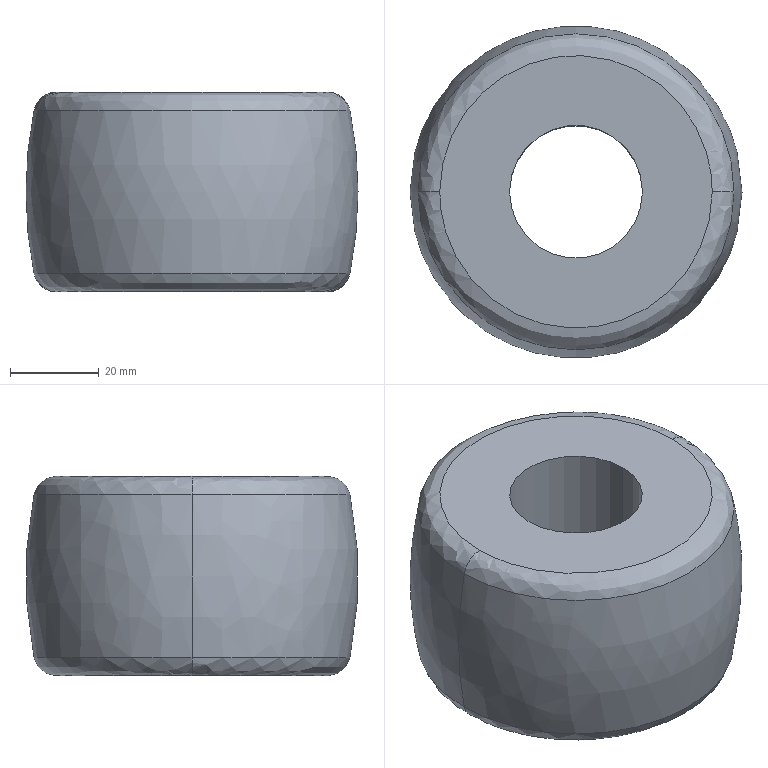Part | STEP file | CDAN75-Mw | 1 solid | 10 faces | box 75 x 74.925 x 45 mm | volume 156321 mm3 | spline 6 | cylinder 2 | plane 2 | commonest cylinder face diameters 30 x2
STEP:
#1=CARTESIAN_POINT('',(0.,0.,0.));
#2=DIRECTION('',(0.,0.,1.));
#3=DIRECTION('',(1.,0.,0.));
#4=AXIS2_PLACEMENT_3D('',#1,#2,#3);
#5=CARTESIAN_POINT('',(-20.313,-59.,18.472));
#6=VERTEX_POINT('',#5);
#7=CARTESIAN_POINT('',(-91.687,-59.,18.472));
#8=VERTEX_POINT('',#7);
#9=CARTESIAN_POINT('',(-56.,-59.,18.472));
#10=DIRECTION('',(0.,0.,-1.));
#11=DIRECTION('',(1.,0.,0.));
#12=AXIS2_PLACEMENT_3D('',#9,#10,#11);
#13=CIRCLE('',#12,35.687);
#14=CARTESIAN_POINT('',(-91.687,-59.,18.472));
#15=CARTESIAN_POINT('',(-91.687,-130.374,18.472));
#16=CARTESIAN_POINT('',(-20.313,-130.374,18.472));
#17=CARTESIAN_POINT('',(-20.313,-59.,18.472));
#18=CARTESIAN_POINT('',(-94.112,-59.,6.237));
#19=CARTESIAN_POINT('',(-94.112,-135.224,6.237));
#20=CARTESIAN_POINT('',(-17.888,-135.224,6.237));
#21=CARTESIAN_POINT('',(-17.888,-59.,6.237));
#22=CARTESIAN_POINT('',(-94.112,-59.,-6.237));
#23=CARTESIAN_POINT('',(-94.112,-135.224,-6.237));
#24=CARTESIAN_POINT('',(-17.888,-135.224,-6.237));
#25=CARTESIAN_POINT('',(-17.888,-59.,-6.237));
#26=CARTESIAN_POINT('',(-91.687,-59.,-18.472));
#27=CARTESIAN_POINT('',(-91.687,-130.374,-18.472));
#28=CARTESIAN_POINT('',(-20.313,-130.374,-18.472));
#29=CARTESIAN_POINT('',(-20.313,-59.,-18.472));
#30=(BOUNDED_SURFACE()B_SPLINE_SURFACE(3,3,((#14,#15,#16,#17),(#18,#19,#20,#21),(#22,#23,#24,#25),(#26,#27,#28,#29)),.UNSPECIFIED.,.F.,.F.,.F.)B_SPLINE_SURFACE_WITH_KNOTS((4,4),(4,4),(0.,1.),(0.,1.),.PIECEWISE_BEZIER_KNOTS.)GEOMETRIC_REPRESENTATION_ITEM()RATIONAL_B_SPLINE_SURFACE(((1.,0.3333,0.3333,1.),(0.9873,0.3291,0.3291,0.9873),(0.9873,0.3291,0.3291,0.9873),(1.,0.3333,0.3333,1.)))REPRESENTATION_ITEM('')SURFACE());
#31=CARTESIAN_POINT('',(0.,1.));
#32=CARTESIAN_POINT('',(0.,0.9763));
#33=CARTESIAN_POINT('',(0.,0.9319));
#34=CARTESIAN_POINT('',(0.,0.8733));
#35=CARTESIAN_POINT('',(0.,0.8206));
#36=CARTESIAN_POINT('',(0.,0.7724));
#37=CARTESIAN_POINT('',(0.,0.7279));
#38=CARTESIAN_POINT('',(0.,0.6861));
#39=CARTESIAN_POINT('',(0.,0.6465));
#40=CARTESIAN_POINT('',(0.,0.6086));
#41=CARTESIAN_POINT('',(0.,0.5718));
#42=CARTESIAN_POINT('',(0.,0.5357));
#43=CARTESIAN_POINT('',(0.,0.5));
#44=CARTESIAN_POINT('',(0.,0.4643));
#45=CARTESIAN_POINT('',(0.,0.4282));
#46=CARTESIAN_POINT('',(0.,0.3914));
#47=CARTESIAN_POINT('',(0.,0.3535));
#48=CARTESIAN_POINT('',(0.,0.3139));
#49=CARTESIAN_POINT('',(0.,0.2721));
#50=CARTESIAN_POINT('',(0.,0.2276));
#51=CARTESIAN_POINT('',(0.,0.1794));
#52=CARTESIAN_POINT('',(0.,0.1267));
#53=CARTESIAN_POINT('',(0.,0.06805));
#54=CARTESIAN_POINT('',(0.,0.02375));
#55=CARTESIAN_POINT('',(0.,0.));
#56=B_SPLINE_CURVE_WITH_KNOTS('',3,(#31,#32,#33,#34,#35,#36,#37,#38,#39,#40,#41,#42,#43,#44,#45,#46,#47,#48,#49,#50,#51,#52,#53,#54,#55),.UNSPECIFIED.,.F.,.F.,(4,1,1,1,1,1,1,1,1,1,1,1,1,1,1,1,1,1,1,1,1,1,4),(0.,0.1428,0.2856,0.4284,0.5712,0.714,0.8568,0.9996,1.142,1.285,1.428,1.571,1.714,1.856,1.999,2.142,2.285,2.428,2.57,2.713,2.856,2.999,3.142),.QUASI_UNIFORM_KNOTS.);
#57=(GEOMETRIC_REPRESENTATION_CONTEXT(2)PARAMETRIC_REPRESENTATION_CONTEXT()REPRESENTATION_CONTEXT('',''));
#58=DEFINITIONAL_REPRESENTATION('',(#56),#57);
#59=PCURVE('',#30,#58);
#60=CARTESIAN_POINT('',(-86.782,-59.,22.5));
#61=CARTESIAN_POINT('',(-86.782,-120.564,22.5));
#62=CARTESIAN_POINT('',(-25.218,-120.564,22.5));
#63=CARTESIAN_POINT('',(-25.218,-59.,22.5));
#64=CARTESIAN_POINT('',(-89.275,-59.,22.5));
#65=CARTESIAN_POINT('',(-89.275,-125.551,22.5));
#66=CARTESIAN_POINT('',(-22.725,-125.551,22.5));
#67=CARTESIAN_POINT('',(-22.725,-59.,22.5));
#68=CARTESIAN_POINT('',(-91.202,-59.,20.918));
#69=CARTESIAN_POINT('',(-91.202,-129.404,20.918));
#70=CARTESIAN_POINT('',(-20.798,-129.404,20.918));
#71=CARTESIAN_POINT('',(-20.798,-59.,20.918));
#72=CARTESIAN_POINT('',(-91.687,-59.,18.472));
#73=CARTESIAN_POINT('',(-91.687,-130.374,18.472));
#74=CARTESIAN_POINT('',(-20.313,-130.374,18.472));
#75=CARTESIAN_POINT('',(-20.313,-59.,18.472));
#76=(BOUNDED_SURFACE()B_SPLINE_SURFACE(3,3,((#60,#61,#62,#63),(#64,#65,#66,#67),(#68,#69,#70,#71),(#72,#73,#74,#75)),.UNSPECIFIED.,.F.,.F.,.F.)B_SPLINE_SURFACE_WITH_KNOTS((4,4),(4,4),(0.,1.),(0.,1.),.PIECEWISE_BEZIER_KNOTS.)GEOMETRIC_REPRESENTATION_ITEM()RATIONAL_B_SPLINE_SURFACE(((1.,0.3333,0.3333,1.),(0.8485,0.2828,0.2828,0.8485),(0.8485,0.2828,0.2828,0.8485),(1.,0.3333,0.3333,1.)))REPRESENTATION_ITEM('')SURFACE());
#77=CARTESIAN_POINT('',(1.,1.));
#78=CARTESIAN_POINT('',(1.,0.9763));
#79=CARTESIAN_POINT('',(1.,0.9319));
#80=CARTESIAN_POINT('',(1.,0.8733));
#81=CARTESIAN_POINT('',(1.,0.8206));
#82=CARTESIAN_POINT('',(1.,0.7724));
#83=CARTESIAN_POINT('',(1.,0.7279));
#84=CARTESIAN_POINT('',(1.,0.6861));
#85=CARTESIAN_POINT('',(1.,0.6465));
#86=CARTESIAN_POINT('',(1.,0.6086));
#87=CARTESIAN_POINT('',(1.,0.5718));
#88=CARTESIAN_POINT('',(1.,0.5357));
#89=CARTESIAN_POINT('',(1.,0.5));
#90=CARTESIAN_POINT('',(1.,0.4643));
#91=CARTESIAN_POINT('',(1.,0.4282));
#92=CARTESIAN_POINT('',(1.,0.3914));
#93=CARTESIAN_POINT('',(1.,0.3535));
#94=CARTESIAN_POINT('',(1.,0.3139));
#95=CARTESIAN_POINT('',(1.,0.2721));
#96=CARTESIAN_POINT('',(1.,0.2276));
#97=CARTESIAN_POINT('',(1.,0.1794));
#98=CARTESIAN_POINT('',(1.,0.1267));
#99=CARTESIAN_POINT('',(1.,0.06805));
#100=CARTESIAN_POINT('',(1.,0.02375));
#101=CARTESIAN_POINT('',(1.,0.));
#102=B_SPLINE_CURVE_WITH_KNOTS('',3,(#77,#78,#79,#80,#81,#82,#83,#84,#85,#86,#87,#88,#89,#90,#91,#92,#93,#94,#95,#96,#97,#98,#99,#100,#101),.UNSPECIFIED.,.F.,.F.,(4,1,1,1,1,1,1,1,1,1,1,1,1,1,1,1,1,1,1,1,1,1,4),(0.,0.1428,0.2856,0.4284,0.5712,0.714,0.8568,0.9996,1.142,1.285,1.428,1.571,1.714,1.856,1.999,2.142,2.285,2.428,2.57,2.713,2.856,2.999,3.142),.QUASI_UNIFORM_KNOTS.);
#103=(GEOMETRIC_REPRESENTATION_CONTEXT(2)PARAMETRIC_REPRESENTATION_CONTEXT()REPRESENTATION_CONTEXT('',''));
#104=DEFINITIONAL_REPRESENTATION('',(#102),#103);
#105=PCURVE('',#76,#104);
#106=SURFACE_CURVE('',#13,(#59,#105),.PCURVE_S1.);
#107=EDGE_CURVE('',#6,#8,#106,.T.);
#108=ORIENTED_EDGE('',*,*,#107,.T.);
#109=CARTESIAN_POINT('',(-91.687,-59.,-18.472));
#110=VERTEX_POINT('',#109);
#111=CARTESIAN_POINT('',(1.5,-59.,0.));
#112=DIRECTION('',(0.,-1.,0.));
#113=DIRECTION('',(-1.,0.,0.));
#114=AXIS2_PLACEMENT_3D('',#111,#112,#113);
#115=CIRCLE('',#114,95.);
#116=CARTESIAN_POINT('',(0.,0.));
#117=CARTESIAN_POINT('',(0.01525,0.));
#118=CARTESIAN_POINT('',(0.04572,0.));
#119=CARTESIAN_POINT('',(0.09135,0.));
#120=CARTESIAN_POINT('',(0.1369,0.));
#121=CARTESIAN_POINT('',(0.1824,0.));
#122=CARTESIAN_POINT('',(0.2279,0.));
#123=CARTESIAN_POINT('',(0.2733,0.));
#124=CARTESIAN_POINT('',(0.3187,0.));
#125=CARTESIAN_POINT('',(0.364,0.));
#126=CARTESIAN_POINT('',(0.4094,0.));
#127=CARTESIAN_POINT('',(0.4547,0.));
#128=CARTESIAN_POINT('',(0.5,0.));
#129=CARTESIAN_POINT('',(0.5453,0.));
#130=CARTESIAN_POINT('',(0.5906,0.));
#131=CARTESIAN_POINT('',(0.636,0.));
#132=CARTESIAN_POINT('',(0.6813,0.));
#133=CARTESIAN_POINT('',(0.7267,0.));
#134=CARTESIAN_POINT('',(0.7721,0.));
#135=CARTESIAN_POINT('',(0.8176,0.));
#136=CARTESIAN_POINT('',(0.8631,0.));
#137=CARTESIAN_POINT('',(0.9086,0.));
#138=CARTESIAN_POINT('',(0.9543,0.));
#139=CARTESIAN_POINT('',(0.9848,0.));
#140=CARTESIAN_POINT('',(1.,0.));
#141=B_SPLINE_CURVE_WITH_KNOTS('',3,(#116,#117,#118,#119,#120,#121,#122,#123,#124,#125,#126,#127,#128,#129,#130,#131,#132,#133,#134,#135,#136,#137,#138,#139,#140),.UNSPECIFIED.,.F.,.F.,(4,1,1,1,1,1,1,1,1,1,1,1,1,1,1,1,1,1,1,1,1,1,4),(6.087,6.105,6.123,6.141,6.159,6.176,6.194,6.212,6.23,6.248,6.265,6.283,6.301,6.319,6.337,6.354,6.372,6.39,6.408,6.426,6.443,6.461,6.479),.QUASI_UNIFORM_KNOTS.);
#142=(GEOMETRIC_REPRESENTATION_CONTEXT(2)PARAMETRIC_REPRESENTATION_CONTEXT()REPRESENTATION_CONTEXT('',''));
#143=DEFINITIONAL_REPRESENTATION('',(#141),#142);
#144=PCURVE('',#30,#143);
#145=CARTESIAN_POINT('',(-20.313,-59.,18.472));
#146=CARTESIAN_POINT('',(-20.313,12.374,18.472));
#147=CARTESIAN_POINT('',(-91.687,12.374,18.472));
#148=CARTESIAN_POINT('',(-91.687,-59.,18.472));
#149=CARTESIAN_POINT('',(-17.888,-59.,6.237));
#150=CARTESIAN_POINT('',(-17.888,17.224,6.237));
#151=CARTESIAN_POINT('',(-94.112,17.224,6.237));
#152=CARTESIAN_POINT('',(-94.112,-59.,6.237));
#153=CARTESIAN_POINT('',(-17.888,-59.,-6.237));
#154=CARTESIAN_POINT('',(-17.888,17.224,-6.237));
#155=CARTESIAN_POINT('',(-94.112,17.224,-6.237));
#156=CARTESIAN_POINT('',(-94.112,-59.,-6.237));
#157=CARTESIAN_POINT('',(-20.313,-59.,-18.472));
#158=CARTESIAN_POINT('',(-20.313,12.374,-18.472));
#159=CARTESIAN_POINT('',(-91.687,12.374,-18.472));
#160=CARTESIAN_POINT('',(-91.687,-59.,-18.472));
#161=(BOUNDED_SURFACE()B_SPLINE_SURFACE(3,3,((#145,#146,#147,#148),(#149,#150,#151,#152),(#153,#154,#155,#156),(#157,#158,#159,#160)),.UNSPECIFIED.,.F.,.F.,.F.)B_SPLINE_SURFACE_WITH_KNOTS((4,4),(4,4),(0.,1.),(0.,1.),.PIECEWISE_BEZIER_KNOTS.)GEOMETRIC_REPRESENTATION_ITEM()RATIONAL_B_SPLINE_SURFACE(((1.,0.3333,0.3333,1.),(0.9873,0.3291,0.3291,0.9873),(0.9873,0.3291,0.3291,0.9873),(1.,0.3333,0.3333,1.)))REPRESENTATION_ITEM('')SURFACE());
#162=CARTESIAN_POINT('',(0.,1.));
#163=CARTESIAN_POINT('',(0.01525,1.));
#164=CARTESIAN_POINT('',(0.04572,1.));
#165=CARTESIAN_POINT('',(0.09135,1.));
#166=CARTESIAN_POINT('',(0.1369,1.));
#167=CARTESIAN_POINT('',(0.1824,1.));
#168=CARTESIAN_POINT('',(0.2279,1.));
#169=CARTESIAN_POINT('',(0.2733,1.));
#170=CARTESIAN_POINT('',(0.3187,1.));
#171=CARTESIAN_POINT('',(0.364,1.));
#172=CARTESIAN_POINT('',(0.4094,1.));
#173=CARTESIAN_POINT('',(0.4547,1.));
#174=CARTESIAN_POINT('',(0.5,1.));
#175=CARTESIAN_POINT('',(0.5453,1.));
#176=CARTESIAN_POINT('',(0.5906,1.));
#177=CARTESIAN_POINT('',(0.636,1.));
#178=CARTESIAN_POINT('',(0.6813,1.));
#179=CARTESIAN_POINT('',(0.7267,1.));
#180=CARTESIAN_POINT('',(0.7721,1.));
#181=CARTESIAN_POINT('',(0.8176,1.));
#182=CARTESIAN_POINT('',(0.8631,1.));
#183=CARTESIAN_POINT('',(0.9086,1.));
#184=CARTESIAN_POINT('',(0.9543,1.));
#185=CARTESIAN_POINT('',(0.9848,1.));
#186=CARTESIAN_POINT('',(1.,1.));
#187=B_SPLINE_CURVE_WITH_KNOTS('',3,(#162,#163,#164,#165,#166,#167,#168,#169,#170,#171,#172,#173,#174,#175,#176,#177,#178,#179,#180,#181,#182,#183,#184,#185,#186),.UNSPECIFIED.,.F.,.F.,(4,1,1,1,1,1,1,1,1,1,1,1,1,1,1,1,1,1,1,1,1,1,4),(6.087,6.105,6.123,6.141,6.159,6.176,6.194,6.212,6.23,6.248,6.265,6.283,6.301,6.319,6.337,6.354,6.372,6.39,6.408,6.426,6.443,6.461,6.479),.QUASI_UNIFORM_KNOTS.);
#188=(GEOMETRIC_REPRESENTATION_CONTEXT(2)PARAMETRIC_REPRESENTATION_CONTEXT()REPRESENTATION_CONTEXT('',''));
#189=DEFINITIONAL_REPRESENTATION('',(#187),#188);
#190=PCURVE('',#161,#189);
#191=SURFACE_CURVE('',#115,(#144,#190),.PCURVE_S1.);
#192=EDGE_CURVE('',#8,#110,#191,.T.);
#193=ORIENTED_EDGE('',*,*,#192,.T.);
#194=CARTESIAN_POINT('',(-20.313,-59.,-18.472));
#195=VERTEX_POINT('',#194);
#196=CARTESIAN_POINT('',(-56.,-59.,-18.472));
#197=DIRECTION('',(0.,0.,1.));
#198=DIRECTION('',(1.,0.,0.));
#199=AXIS2_PLACEMENT_3D('',#196,#197,#198);
#200=CIRCLE('',#199,35.687);
#201=CARTESIAN_POINT('',(1.,0.));
#202=CARTESIAN_POINT('',(1.,0.02375));
#203=CARTESIAN_POINT('',(1.,0.06805));
#204=CARTESIAN_POINT('',(1.,0.1267));
#205=CARTESIAN_POINT('',(1.,0.1794));
#206=CARTESIAN_POINT('',(1.,0.2276));
#207=CARTESIAN_POINT('',(1.,0.2721));
#208=CARTESIAN_POINT('',(1.,0.3139));
#209=CARTESIAN_POINT('',(1.,0.3535));
#210=CARTESIAN_POINT('',(1.,0.3914));
#211=CARTESIAN_POINT('',(1.,0.4282));
#212=CARTESIAN_POINT('',(1.,0.4643));
#213=CARTESIAN_POINT('',(1.,0.5));
#214=CARTESIAN_POINT('',(1.,0.5357));
#215=CARTESIAN_POINT('',(1.,0.5718));
#216=CARTESIAN_POINT('',(1.,0.6086));
#217=CARTESIAN_POINT('',(1.,0.6465));
#218=CARTESIAN_POINT('',(1.,0.6861));
#219=CARTESIAN_POINT('',(1.,0.7279));
#220=CARTESIAN_POINT('',(1.,0.7724));
#221=CARTESIAN_POINT('',(1.,0.8206));
#222=CARTESIAN_POINT('',(1.,0.8733));
#223=CARTESIAN_POINT('',(1.,0.9319));
#224=CARTESIAN_POINT('',(1.,0.9763));
#225=CARTESIAN_POINT('',(1.,1.));
#226=B_SPLINE_CURVE_WITH_KNOTS('',3,(#201,#202,#203,#204,#205,#206,#207,#208,#209,#210,#211,#212,#213,#214,#215,#216,#217,#218,#219,#220,#221,#222,#223,#224,#225),.UNSPECIFIED.,.F.,.F.,(4,1,1,1,1,1,1,1,1,1,1,1,1,1,1,1,1,1,1,1,1,1,4),(3.142,3.284,3.427,3.57,3.713,3.856,3.998,4.141,4.284,4.427,4.57,4.712,4.855,4.998,5.141,5.284,5.426,5.569,5.712,5.855,5.998,6.14,6.283),.QUASI_UNIFORM_KNOTS.);
#227=(GEOMETRIC_REPRESENTATION_CONTEXT(2)PARAMETRIC_REPRESENTATION_CONTEXT()REPRESENTATION_CONTEXT('',''));
#228=DEFINITIONAL_REPRESENTATION('',(#226),#227);
#229=PCURVE('',#30,#228);
#230=CARTESIAN_POINT('',(-91.687,-59.,-18.472));
#231=CARTESIAN_POINT('',(-91.687,-130.374,-18.472));
#232=CARTESIAN_POINT('',(-20.313,-130.374,-18.472));
#233=CARTESIAN_POINT('',(-20.313,-59.,-18.472));
#234=CARTESIAN_POINT('',(-91.202,-59.,-20.918));
#235=CARTESIAN_POINT('',(-91.202,-129.404,-20.918));
#236=CARTESIAN_POINT('',(-20.798,-129.404,-20.918));
#237=CARTESIAN_POINT('',(-20.798,-59.,-20.918));
#238=CARTESIAN_POINT('',(-89.275,-59.,-22.5));
#239=CARTESIAN_POINT('',(-89.275,-125.551,-22.5));
#240=CARTESIAN_POINT('',(-22.725,-125.551,-22.5));
#241=CARTESIAN_POINT('',(-22.725,-59.,-22.5));
#242=CARTESIAN_POINT('',(-86.782,-59.,-22.5));
#243=CARTESIAN_POINT('',(-86.782,-120.564,-22.5));
#244=CARTESIAN_POINT('',(-25.218,-120.564,-22.5));
#245=CARTESIAN_POINT('',(-25.218,-59.,-22.5));
#246=(BOUNDED_SURFACE()B_SPLINE_SURFACE(3,3,((#230,#231,#232,#233),(#234,#235,#236,#237),(#238,#239,#240,#241),(#242,#243,#244,#245)),.UNSPECIFIED.,.F.,.F.,.F.)B_SPLINE_SURFACE_WITH_KNOTS((4,4),(4,4),(0.,1.),(0.,1.),.PIECEWISE_BEZIER_KNOTS.)GEOMETRIC_REPRESENTATION_ITEM()RATIONAL_B_SPLINE_SURFACE(((1.,0.3333,0.3333,1.),(0.8485,0.2828,0.2828,0.8485),(0.8485,0.2828,0.2828,0.8485),(1.,0.3333,0.3333,1.)))REPRESENTATION_ITEM('')SURFACE());
#247=CARTESIAN_POINT('',(0.,0.));
#248=CARTESIAN_POINT('',(0.,0.02375));
#249=CARTESIAN_POINT('',(0.,0.06805));
#250=CARTESIAN_POINT('',(0.,0.1267));
#251=CARTESIAN_POINT('',(0.,0.1794));
#252=CARTESIAN_POINT('',(0.,0.2276));
#253=CARTESIAN_POINT('',(0.,0.2721));
#254=CARTESIAN_POINT('',(0.,0.3139));
#255=CARTESIAN_POINT('',(0.,0.3535));
#256=CARTESIAN_POINT('',(0.,0.3914));
#257=CARTESIAN_POINT('',(0.,0.4282));
#258=CARTESIAN_POINT('',(0.,0.4643));
#259=CARTESIAN_POINT('',(0.,0.5));
#260=CARTESIAN_POINT('',(0.,0.5357));
#261=CARTESIAN_POINT('',(0.,0.5718));
#262=CARTESIAN_POINT('',(0.,0.6086));
#263=CARTESIAN_POINT('',(0.,0.6465));
#264=CARTESIAN_POINT('',(0.,0.6861));
#265=CARTESIAN_POINT('',(0.,0.7279));
#266=CARTESIAN_POINT('',(0.,0.7724));
#267=CARTESIAN_POINT('',(0.,0.8206));
#268=CARTESIAN_POINT('',(0.,0.8733));
#269=CARTESIAN_POINT('',(0.,0.9319));
#270=CARTESIAN_POINT('',(0.,0.9763));
#271=CARTESIAN_POINT('',(0.,1.));
#272=B_SPLINE_CURVE_WITH_KNOTS('',3,(#247,#248,#249,#250,#251,#252,#253,#254,#255,#256,#257,#258,#259,#260,#261,#262,#263,#264,#265,#266,#267,#268,#269,#270,#271),.UNSPECIFIED.,.F.,.F.,(4,1,1,1,1,1,1,1,1,1,1,1,1,1,1,1,1,1,1,1,1,1,4),(3.142,3.284,3.427,3.57,3.713,3.856,3.998,4.141,4.284,4.427,4.57,4.712,4.855,4.998,5.141,5.284,5.426,5.569,5.712,5.855,5.998,6.14,6.283),.QUASI_UNIFORM_KNOTS.);
#273=(GEOMETRIC_REPRESENTATION_CONTEXT(2)PARAMETRIC_REPRESENTATION_CONTEXT()REPRESENTATION_CONTEXT('',''));
#274=DEFINITIONAL_REPRESENTATION('',(#272),#273);
#275=PCURVE('',#246,#274);
#276=SURFACE_CURVE('',#200,(#229,#275),.PCURVE_S1.);
#277=EDGE_CURVE('',#110,#195,#276,.T.);
#278=ORIENTED_EDGE('',*,*,#277,.T.);
#279=CARTESIAN_POINT('',(-113.5,-59.,0.));
#280=DIRECTION('',(0.,1.,0.));
#281=DIRECTION('',(1.,0.,0.));
#282=AXIS2_PLACEMENT_3D('',#279,#280,#281);
#283=CIRCLE('',#282,95.);
#284=CARTESIAN_POINT('',(0.,1.));
#285=CARTESIAN_POINT('',(0.01525,1.));
#286=CARTESIAN_POINT('',(0.04572,1.));
#287=CARTESIAN_POINT('',(0.09135,1.));
#288=CARTESIAN_POINT('',(0.1369,1.));
#289=CARTESIAN_POINT('',(0.1824,1.));
#290=CARTESIAN_POINT('',(0.2279,1.));
#291=CARTESIAN_POINT('',(0.2733,1.));
#292=CARTESIAN_POINT('',(0.3187,1.));
#293=CARTESIAN_POINT('',(0.364,1.));
#294=CARTESIAN_POINT('',(0.4094,1.));
#295=CARTESIAN_POINT('',(0.4547,1.));
#296=CARTESIAN_POINT('',(0.5,1.));
#297=CARTESIAN_POINT('',(0.5453,1.));
#298=CARTESIAN_POINT('',(0.5906,1.));
#299=CARTESIAN_POINT('',(0.636,1.));
#300=CARTESIAN_POINT('',(0.6813,1.));
#301=CARTESIAN_POINT('',(0.7267,1.));
#302=CARTESIAN_POINT('',(0.7721,1.));
#303=CARTESIAN_POINT('',(0.8176,1.));
#304=CARTESIAN_POINT('',(0.8631,1.));
#305=CARTESIAN_POINT('',(0.9086,1.));
#306=CARTESIAN_POINT('',(0.9543,1.));
#307=CARTESIAN_POINT('',(0.9848,1.));
#308=CARTESIAN_POINT('',(1.,1.));
#309=B_SPLINE_CURVE_WITH_KNOTS('',3,(#284,#285,#286,#287,#288,#289,#290,#291,#292,#293,#294,#295,#296,#297,#298,#299,#300,#301,#302,#303,#304,#305,#306,#307,#308),.UNSPECIFIED.,.F.,.F.,(4,1,1,1,1,1,1,1,1,1,1,1,1,1,1,1,1,1,1,1,1,1,4),(6.087,6.105,6.123,6.141,6.159,6.176,6.194,6.212,6.23,6.248,6.265,6.283,6.301,6.319,6.337,6.354,6.372,6.39,6.408,6.426,6.443,6.461,6.479),.QUASI_UNIFORM_KNOTS.);
#310=(GEOMETRIC_REPRESENTATION_CONTEXT(2)PARAMETRIC_REPRESENTATION_CONTEXT()REPRESENTATION_CONTEXT('',''));
#311=DEFINITIONAL_REPRESENTATION('',(#309),#310);
#312=PCURVE('',#30,#311);
#313=CARTESIAN_POINT('',(0.,0.));
#314=CARTESIAN_POINT('',(0.01525,0.));
#315=CARTESIAN_POINT('',(0.04572,0.));
#316=CARTESIAN_POINT('',(0.09135,0.));
#317=CARTESIAN_POINT('',(0.1369,0.));
#318=CARTESIAN_POINT('',(0.1824,0.));
#319=CARTESIAN_POINT('',(0.2279,0.));
#320=CARTESIAN_POINT('',(0.2733,0.));
#321=CARTESIAN_POINT('',(0.3187,0.));
#322=CARTESIAN_POINT('',(0.364,0.));
#323=CARTESIAN_POINT('',(0.4094,0.));
#324=CARTESIAN_POINT('',(0.4547,0.));
#325=CARTESIAN_POINT('',(0.5,0.));
#326=CARTESIAN_POINT('',(0.5453,0.));
#327=CARTESIAN_POINT('',(0.5906,0.));
#328=CARTESIAN_POINT('',(0.636,0.));
#329=CARTESIAN_POINT('',(0.6813,0.));
#330=CARTESIAN_POINT('',(0.7267,0.));
#331=CARTESIAN_POINT('',(0.7721,0.));
#332=CARTESIAN_POINT('',(0.8176,0.));
#333=CARTESIAN_POINT('',(0.8631,0.));
#334=CARTESIAN_POINT('',(0.9086,0.));
#335=CARTESIAN_POINT('',(0.9543,0.));
#336=CARTESIAN_POINT('',(0.9848,0.));
#337=CARTESIAN_POINT('',(1.,0.));
#338=B_SPLINE_CURVE_WITH_KNOTS('',3,(#313,#314,#315,#316,#317,#318,#319,#320,#321,#322,#323,#324,#325,#326,#327,#328,#329,#330,#331,#332,#333,#334,#335,#336,#337),.UNSPECIFIED.,.F.,.F.,(4,1,1,1,1,1,1,1,1,1,1,1,1,1,1,1,1,1,1,1,1,1,4),(6.087,6.105,6.123,6.141,6.159,6.176,6.194,6.212,6.23,6.248,6.265,6.283,6.301,6.319,6.337,6.354,6.372,6.39,6.408,6.426,6.443,6.461,6.479),.QUASI_UNIFORM_KNOTS.);
#339=(GEOMETRIC_REPRESENTATION_CONTEXT(2)PARAMETRIC_REPRESENTATION_CONTEXT()REPRESENTATION_CONTEXT('',''));
#340=DEFINITIONAL_REPRESENTATION('',(#338),#339);
#341=PCURVE('',#161,#340);
#342=SURFACE_CURVE('',#283,(#312,#341),.PCURVE_S1.);
#343=EDGE_CURVE('',#6,#195,#342,.T.);
#344=ORIENTED_EDGE('',*,*,#343,.F.);
#345=EDGE_LOOP('',(#108,#193,#278,#344));
#346=FACE_BOUND('',#345,.T.);
#347=ADVANCED_FACE('',(#346),#30,.T.);
#348=CARTESIAN_POINT('',(-25.218,-59.,22.5));
#349=VERTEX_POINT('',#348);
#350=CARTESIAN_POINT('',(-86.782,-59.,22.5));
#351=VERTEX_POINT('',#350);
#352=CARTESIAN_POINT('',(-25.218,-59.,22.5));
#353=CARTESIAN_POINT('',(-25.218,-120.564,22.5));
#354=CARTESIAN_POINT('',(-86.782,-120.564,22.5));
#355=CARTESIAN_POINT('',(-86.782,-59.,22.5));
#356=(BOUNDED_CURVE()B_SPLINE_CURVE(3,(#352,#353,#354,#355),.UNSPECIFIED.,.F.,.F.)B_SPLINE_CURVE_WITH_KNOTS((4,4),(0.25,0.75),.PIECEWISE_BEZIER_KNOTS.)CURVE()GEOMETRIC_REPRESENTATION_ITEM()RATIONAL_B_SPLINE_CURVE((1.,0.3333,0.3333,1.))REPRESENTATION_ITEM(''));
#357=CARTESIAN_POINT('',(0.,1.));
#358=CARTESIAN_POINT('',(0.,0.));
#359=B_SPLINE_CURVE_WITH_KNOTS('',1,(#357,#358),.UNSPECIFIED.,.F.,.F.,(2,2),(0.25,0.75),.PIECEWISE_BEZIER_KNOTS.);
#360=(GEOMETRIC_REPRESENTATION_CONTEXT(2)PARAMETRIC_REPRESENTATION_CONTEXT()REPRESENTATION_CONTEXT('',''));
#361=DEFINITIONAL_REPRESENTATION('',(#359),#360);
#362=PCURVE('',#76,#361);
#363=CARTESIAN_POINT('',(-56.,-36.109,22.5));
#364=DIRECTION('',(0.,0.,1.));
#365=DIRECTION('',(0.,-1.,0.));
#366=AXIS2_PLACEMENT_3D('',#363,#364,#365);
#367=PLANE('',#366);
#368=CARTESIAN_POINT('',(22.891,30.782));
#369=CARTESIAN_POINT('',(84.456,30.782));
#370=CARTESIAN_POINT('',(84.456,-30.782));
#371=CARTESIAN_POINT('',(22.891,-30.782));
#372=(BOUNDED_CURVE()B_SPLINE_CURVE(3,(#368,#369,#370,#371),.UNSPECIFIED.,.F.,.F.)B_SPLINE_CURVE_WITH_KNOTS((4,4),(0.25,0.75),.PIECEWISE_BEZIER_KNOTS.)CURVE()GEOMETRIC_REPRESENTATION_ITEM()RATIONAL_B_SPLINE_CURVE((1.,0.3333,0.3333,1.))REPRESENTATION_ITEM(''));
#373=(GEOMETRIC_REPRESENTATION_CONTEXT(2)PARAMETRIC_REPRESENTATION_CONTEXT()REPRESENTATION_CONTEXT('',''));
#374=DEFINITIONAL_REPRESENTATION('',(#372),#373);
#375=PCURVE('',#367,#374);
#376=SURFACE_CURVE('',#356,(#362,#375),.PCURVE_S1.);
#377=EDGE_CURVE('',#349,#351,#376,.T.);
#378=ORIENTED_EDGE('',*,*,#377,.T.);
#379=CARTESIAN_POINT('',(-86.782,-59.,17.5));
#380=DIRECTION('',(0.,-1.,0.));
#381=DIRECTION('',(-1.,0.,0.));
#382=AXIS2_PLACEMENT_3D('',#379,#380,#381);
#383=CIRCLE('',#382,5.);
#384=CARTESIAN_POINT('',(0.,0.));
#385=CARTESIAN_POINT('',(0.01641,0.));
#386=CARTESIAN_POINT('',(0.04888,0.));
#387=CARTESIAN_POINT('',(0.0966,0.));
#388=CARTESIAN_POINT('',(0.1435,0.));
#389=CARTESIAN_POINT('',(0.1896,0.));
#390=CARTESIAN_POINT('',(0.2351,0.));
#391=CARTESIAN_POINT('',(0.28,0.));
#392=CARTESIAN_POINT('',(0.3245,0.));
#393=CARTESIAN_POINT('',(0.3687,0.));
#394=CARTESIAN_POINT('',(0.4126,0.));
#395=CARTESIAN_POINT('',(0.4564,0.));
#396=CARTESIAN_POINT('',(0.5,0.));
#397=CARTESIAN_POINT('',(0.5436,0.));
#398=CARTESIAN_POINT('',(0.5874,0.));
#399=CARTESIAN_POINT('',(0.6313,0.));
#400=CARTESIAN_POINT('',(0.6755,0.));
#401=CARTESIAN_POINT('',(0.72,0.));
#402=CARTESIAN_POINT('',(0.7649,0.));
#403=CARTESIAN_POINT('',(0.8104,0.));
#404=CARTESIAN_POINT('',(0.8565,0.));
#405=CARTESIAN_POINT('',(0.9034,0.));
#406=CARTESIAN_POINT('',(0.9511,0.));
#407=CARTESIAN_POINT('',(0.9836,0.));
#408=CARTESIAN_POINT('',(1.,0.));
#409=B_SPLINE_CURVE_WITH_KNOTS('',3,(#384,#385,#386,#387,#388,#389,#390,#391,#392,#393,#394,#395,#396,#397,#398,#399,#400,#401,#402,#403,#404,#405,#406,#407,#408),.UNSPECIFIED.,.F.,.F.,(4,1,1,1,1,1,1,1,1,1,1,1,1,1,1,1,1,1,1,1,1,1,4),(4.712,4.775,4.837,4.9,4.962,5.025,5.087,5.15,5.212,5.275,5.337,5.4,5.462,5.525,5.587,5.65,5.712,5.775,5.837,5.9,5.962,6.025,6.087),.QUASI_UNIFORM_KNOTS.);
#410=(GEOMETRIC_REPRESENTATION_CONTEXT(2)PARAMETRIC_REPRESENTATION_CONTEXT()REPRESENTATION_CONTEXT('',''));
#411=DEFINITIONAL_REPRESENTATION('',(#409),#410);
#412=PCURVE('',#76,#411);
#413=CARTESIAN_POINT('',(-25.218,-59.,22.5));
#414=CARTESIAN_POINT('',(-25.218,2.564,22.5));
#415=CARTESIAN_POINT('',(-86.782,2.564,22.5));
#416=CARTESIAN_POINT('',(-86.782,-59.,22.5));
#417=CARTESIAN_POINT('',(-22.725,-59.,22.5));
#418=CARTESIAN_POINT('',(-22.725,7.551,22.5));
#419=CARTESIAN_POINT('',(-89.275,7.551,22.5));
#420=CARTESIAN_POINT('',(-89.275,-59.,22.5));
#421=CARTESIAN_POINT('',(-20.798,-59.,20.918));
#422=CARTESIAN_POINT('',(-20.798,11.404,20.918));
#423=CARTESIAN_POINT('',(-91.202,11.404,20.918));
#424=CARTESIAN_POINT('',(-91.202,-59.,20.918));
#425=CARTESIAN_POINT('',(-20.313,-59.,18.472));
#426=CARTESIAN_POINT('',(-20.313,12.374,18.472));
#427=CARTESIAN_POINT('',(-91.687,12.374,18.472));
#428=CARTESIAN_POINT('',(-91.687,-59.,18.472));
#429=(BOUNDED_SURFACE()B_SPLINE_SURFACE(3,3,((#413,#414,#415,#416),(#417,#418,#419,#420),(#421,#422,#423,#424),(#425,#426,#427,#428)),.UNSPECIFIED.,.F.,.F.,.F.)B_SPLINE_SURFACE_WITH_KNOTS((4,4),(4,4),(0.,1.),(0.,1.),.PIECEWISE_BEZIER_KNOTS.)GEOMETRIC_REPRESENTATION_ITEM()RATIONAL_B_SPLINE_SURFACE(((1.,0.3333,0.3333,1.),(0.8485,0.2828,0.2828,0.8485),(0.8485,0.2828,0.2828,0.8485),(1.,0.3333,0.3333,1.)))REPRESENTATION_ITEM('')SURFACE());
#430=CARTESIAN_POINT('',(0.,1.));
#431=CARTESIAN_POINT('',(0.01641,1.));
#432=CARTESIAN_POINT('',(0.04888,1.));
#433=CARTESIAN_POINT('',(0.0966,1.));
#434=CARTESIAN_POINT('',(0.1435,1.));
#435=CARTESIAN_POINT('',(0.1896,1.));
#436=CARTESIAN_POINT('',(0.2351,1.));
#437=CARTESIAN_POINT('',(0.28,1.));
#438=CARTESIAN_POINT('',(0.3245,1.));
#439=CARTESIAN_POINT('',(0.3687,1.));
#440=CARTESIAN_POINT('',(0.4126,1.));
#441=CARTESIAN_POINT('',(0.4564,1.));
#442=CARTESIAN_POINT('',(0.5,1.));
#443=CARTESIAN_POINT('',(0.5436,1.));
#444=CARTESIAN_POINT('',(0.5874,1.));
#445=CARTESIAN_POINT('',(0.6313,1.));
#446=CARTESIAN_POINT('',(0.6755,1.));
#447=CARTESIAN_POINT('',(0.72,1.));
#448=CARTESIAN_POINT('',(0.7649,1.));
#449=CARTESIAN_POINT('',(0.8104,1.));
#450=CARTESIAN_POINT('',(0.8565,1.));
#451=CARTESIAN_POINT('',(0.9034,1.));
#452=CARTESIAN_POINT('',(0.9511,1.));
#453=CARTESIAN_POINT('',(0.9836,1.));
#454=CARTESIAN_POINT('',(1.,1.));
#455=B_SPLINE_CURVE_WITH_KNOTS('',3,(#430,#431,#432,#433,#434,#435,#436,#437,#438,#439,#440,#441,#442,#443,#444,#445,#446,#447,#448,#449,#450,#451,#452,#453,#454),.UNSPECIFIED.,.F.,.F.,(4,1,1,1,1,1,1,1,1,1,1,1,1,1,1,1,1,1,1,1,1,1,4),(4.712,4.775,4.837,4.9,4.962,5.025,5.087,5.15,5.212,5.275,5.337,5.4,5.462,5.525,5.587,5.65,5.712,5.775,5.837,5.9,5.962,6.025,6.087),.QUASI_UNIFORM_KNOTS.);
#456=(GEOMETRIC_REPRESENTATION_CONTEXT(2)PARAMETRIC_REPRESENTATION_CONTEXT()REPRESENTATION_CONTEXT('',''));
#457=DEFINITIONAL_REPRESENTATION('',(#455),#456);
#458=PCURVE('',#429,#457);
#459=SURFACE_CURVE('',#383,(#412,#458),.PCURVE_S1.);
#460=EDGE_CURVE('',#351,#8,#459,.T.);
#461=ORIENTED_EDGE('',*,*,#460,.T.);
#462=ORIENTED_EDGE('',*,*,#107,.F.);
#463=CARTESIAN_POINT('',(-25.218,-59.,17.5));
#464=DIRECTION('',(0.,1.,0.));
#465=DIRECTION('',(1.,0.,0.));
#466=AXIS2_PLACEMENT_3D('',#463,#464,#465);
#467=CIRCLE('',#466,5.);
#468=CARTESIAN_POINT('',(0.,1.));
#469=CARTESIAN_POINT('',(0.01641,1.));
#470=CARTESIAN_POINT('',(0.04888,1.));
#471=CARTESIAN_POINT('',(0.0966,1.));
#472=CARTESIAN_POINT('',(0.1435,1.));
#473=CARTESIAN_POINT('',(0.1896,1.));
#474=CARTESIAN_POINT('',(0.2351,1.));
#475=CARTESIAN_POINT('',(0.28,1.));
#476=CARTESIAN_POINT('',(0.3245,1.));
#477=CARTESIAN_POINT('',(0.3687,1.));
#478=CARTESIAN_POINT('',(0.4126,1.));
#479=CARTESIAN_POINT('',(0.4564,1.));
#480=CARTESIAN_POINT('',(0.5,1.));
#481=CARTESIAN_POINT('',(0.5436,1.));
#482=CARTESIAN_POINT('',(0.5874,1.));
#483=CARTESIAN_POINT('',(0.6313,1.));
#484=CARTESIAN_POINT('',(0.6755,1.));
#485=CARTESIAN_POINT('',(0.72,1.));
#486=CARTESIAN_POINT('',(0.7649,1.));
#487=CARTESIAN_POINT('',(0.8104,1.));
#488=CARTESIAN_POINT('',(0.8565,1.));
#489=CARTESIAN_POINT('',(0.9034,1.));
#490=CARTESIAN_POINT('',(0.9511,1.));
#491=CARTESIAN_POINT('',(0.9836,1.));
#492=CARTESIAN_POINT('',(1.,1.));
#493=B_SPLINE_CURVE_WITH_KNOTS('',3,(#468,#469,#470,#471,#472,#473,#474,#475,#476,#477,#478,#479,#480,#481,#482,#483,#484,#485,#486,#487,#488,#489,#490,#491,#492),.UNSPECIFIED.,.F.,.F.,(4,1,1,1,1,1,1,1,1,1,1,1,1,1,1,1,1,1,1,1,1,1,4),(4.712,4.775,4.837,4.9,4.962,5.025,5.087,5.15,5.212,5.275,5.337,5.4,5.462,5.525,5.587,5.65,5.712,5.775,5.837,5.9,5.962,6.025,6.087),.QUASI_UNIFORM_KNOTS.);
#494=(GEOMETRIC_REPRESENTATION_CONTEXT(2)PARAMETRIC_REPRESENTATION_CONTEXT()REPRESENTATION_CONTEXT('',''));
#495=DEFINITIONAL_REPRESENTATION('',(#493),#494);
#496=PCURVE('',#76,#495);
#497=CARTESIAN_POINT('',(0.,0.));
#498=CARTESIAN_POINT('',(0.01641,0.));
#499=CARTESIAN_POINT('',(0.04888,0.));
#500=CARTESIAN_POINT('',(0.0966,0.));
#501=CARTESIAN_POINT('',(0.1435,0.));
#502=CARTESIAN_POINT('',(0.1896,0.));
#503=CARTESIAN_POINT('',(0.2351,0.));
#504=CARTESIAN_POINT('',(0.28,0.));
#505=CARTESIAN_POINT('',(0.3245,0.));
#506=CARTESIAN_POINT('',(0.3687,0.));
#507=CARTESIAN_POINT('',(0.4126,0.));
#508=CARTESIAN_POINT('',(0.4564,0.));
#509=CARTESIAN_POINT('',(0.5,0.));
#510=CARTESIAN_POINT('',(0.5436,0.));
#511=CARTESIAN_POINT('',(0.5874,0.));
#512=CARTESIAN_POINT('',(0.6313,0.));
#513=CARTESIAN_POINT('',(0.6755,0.));
#514=CARTESIAN_POINT('',(0.72,0.));
#515=CARTESIAN_POINT('',(0.7649,0.));
#516=CARTESIAN_POINT('',(0.8104,0.));
#517=CARTESIAN_POINT('',(0.8565,0.));
#518=CARTESIAN_POINT('',(0.9034,0.));
#519=CARTESIAN_POINT('',(0.9511,0.));
#520=CARTESIAN_POINT('',(0.9836,0.));
#521=CARTESIAN_POINT('',(1.,0.));
#522=B_SPLINE_CURVE_WITH_KNOTS('',3,(#497,#498,#499,#500,#501,#502,#503,#504,#505,#506,#507,#508,#509,#510,#511,#512,#513,#514,#515,#516,#517,#518,#519,#520,#521),.UNSPECIFIED.,.F.,.F.,(4,1,1,1,1,1,1,1,1,1,1,1,1,1,1,1,1,1,1,1,1,1,4),(4.712,4.775,4.837,4.9,4.962,5.025,5.087,5.15,5.212,5.275,5.337,5.4,5.462,5.525,5.587,5.65,5.712,5.775,5.837,5.9,5.962,6.025,6.087),.QUASI_UNIFORM_KNOTS.);
#523=(GEOMETRIC_REPRESENTATION_CONTEXT(2)PARAMETRIC_REPRESENTATION_CONTEXT()REPRESENTATION_CONTEXT('',''));
#524=DEFINITIONAL_REPRESENTATION('',(#522),#523);
#525=PCURVE('',#429,#524);
#526=SURFACE_CURVE('',#467,(#496,#525),.PCURVE_S1.);
#527=EDGE_CURVE('',#349,#6,#526,.T.);
#528=ORIENTED_EDGE('',*,*,#527,.F.);
#529=EDGE_LOOP('',(#378,#461,#462,#528));
#530=FACE_BOUND('',#529,.T.);
#531=ADVANCED_FACE('',(#530),#76,.T.);
#532=ORIENTED_EDGE('',*,*,#277,.F.);
#533=CARTESIAN_POINT('',(-86.782,-59.,-22.5));
#534=VERTEX_POINT('',#533);
#535=CARTESIAN_POINT('',(-86.782,-59.,-17.5));
#536=DIRECTION('',(0.,-1.,0.));
#537=DIRECTION('',(-1.,0.,0.));
#538=AXIS2_PLACEMENT_3D('',#535,#536,#537);
#539=CIRCLE('',#538,5.);
#540=CARTESIAN_POINT('',(0.,0.));
#541=CARTESIAN_POINT('',(0.01641,0.));
#542=CARTESIAN_POINT('',(0.04888,0.));
#543=CARTESIAN_POINT('',(0.0966,0.));
#544=CARTESIAN_POINT('',(0.1435,0.));
#545=CARTESIAN_POINT('',(0.1896,0.));
#546=CARTESIAN_POINT('',(0.2351,0.));
#547=CARTESIAN_POINT('',(0.28,0.));
#548=CARTESIAN_POINT('',(0.3245,0.));
#549=CARTESIAN_POINT('',(0.3687,0.));
#550=CARTESIAN_POINT('',(0.4126,0.));
#551=CARTESIAN_POINT('',(0.4564,0.));
#552=CARTESIAN_POINT('',(0.5,0.));
#553=CARTESIAN_POINT('',(0.5436,0.));
#554=CARTESIAN_POINT('',(0.5874,0.));
#555=CARTESIAN_POINT('',(0.6313,0.));
#556=CARTESIAN_POINT('',(0.6755,0.));
#557=CARTESIAN_POINT('',(0.72,0.));
#558=CARTESIAN_POINT('',(0.7649,0.));
#559=CARTESIAN_POINT('',(0.8104,0.));
#560=CARTESIAN_POINT('',(0.8565,0.));
#561=CARTESIAN_POINT('',(0.9034,0.));
#562=CARTESIAN_POINT('',(0.9511,0.));
#563=CARTESIAN_POINT('',(0.9836,0.));
#564=CARTESIAN_POINT('',(1.,0.));
#565=B_SPLINE_CURVE_WITH_KNOTS('',3,(#540,#541,#542,#543,#544,#545,#546,#547,#548,#549,#550,#551,#552,#553,#554,#555,#556,#557,#558,#559,#560,#561,#562,#563,#564),.UNSPECIFIED.,.F.,.F.,(4,1,1,1,1,1,1,1,1,1,1,1,1,1,1,1,1,1,1,1,1,1,4),(0.1957,0.2582,0.3207,0.3832,0.4457,0.5082,0.5707,0.6332,0.6957,0.7582,0.8207,0.8832,0.9457,1.008,1.071,1.133,1.196,1.258,1.321,1.383,1.446,1.508,1.571),.QUASI_UNIFORM_KNOTS.);
#566=(GEOMETRIC_REPRESENTATION_CONTEXT(2)PARAMETRIC_REPRESENTATION_CONTEXT()REPRESENTATION_CONTEXT('',''));
#567=DEFINITIONAL_REPRESENTATION('',(#565),#566);
#568=PCURVE('',#246,#567);
#569=CARTESIAN_POINT('',(-20.313,-59.,-18.472));
#570=CARTESIAN_POINT('',(-20.313,12.374,-18.472));
#571=CARTESIAN_POINT('',(-91.687,12.374,-18.472));
#572=CARTESIAN_POINT('',(-91.687,-59.,-18.472));
#573=CARTESIAN_POINT('',(-20.798,-59.,-20.918));
#574=CARTESIAN_POINT('',(-20.798,11.404,-20.918));
#575=CARTESIAN_POINT('',(-91.202,11.404,-20.918));
#576=CARTESIAN_POINT('',(-91.202,-59.,-20.918));
#577=CARTESIAN_POINT('',(-22.725,-59.,-22.5));
#578=CARTESIAN_POINT('',(-22.725,7.551,-22.5));
#579=CARTESIAN_POINT('',(-89.275,7.551,-22.5));
#580=CARTESIAN_POINT('',(-89.275,-59.,-22.5));
#581=CARTESIAN_POINT('',(-25.218,-59.,-22.5));
#582=CARTESIAN_POINT('',(-25.218,2.564,-22.5));
#583=CARTESIAN_POINT('',(-86.782,2.564,-22.5));
#584=CARTESIAN_POINT('',(-86.782,-59.,-22.5));
#585=(BOUNDED_SURFACE()B_SPLINE_SURFACE(3,3,((#569,#570,#571,#572),(#573,#574,#575,#576),(#577,#578,#579,#580),(#581,#582,#583,#584)),.UNSPECIFIED.,.F.,.F.,.F.)B_SPLINE_SURFACE_WITH_KNOTS((4,4),(4,4),(0.,1.),(0.,1.),.PIECEWISE_BEZIER_KNOTS.)GEOMETRIC_REPRESENTATION_ITEM()RATIONAL_B_SPLINE_SURFACE(((1.,0.3333,0.3333,1.),(0.8485,0.2828,0.2828,0.8485),(0.8485,0.2828,0.2828,0.8485),(1.,0.3333,0.3333,1.)))REPRESENTATION_ITEM('')SURFACE());
#586=CARTESIAN_POINT('',(0.,1.));
#587=CARTESIAN_POINT('',(0.01641,1.));
#588=CARTESIAN_POINT('',(0.04888,1.));
#589=CARTESIAN_POINT('',(0.0966,1.));
#590=CARTESIAN_POINT('',(0.1435,1.));
#591=CARTESIAN_POINT('',(0.1896,1.));
#592=CARTESIAN_POINT('',(0.2351,1.));
#593=CARTESIAN_POINT('',(0.28,1.));
#594=CARTESIAN_POINT('',(0.3245,1.));
#595=CARTESIAN_POINT('',(0.3687,1.));
#596=CARTESIAN_POINT('',(0.4126,1.));
#597=CARTESIAN_POINT('',(0.4564,1.));
#598=CARTESIAN_POINT('',(0.5,1.));
#599=CARTESIAN_POINT('',(0.5436,1.));
#600=CARTESIAN_POINT('',(0.5874,1.));
#601=CARTESIAN_POINT('',(0.6313,1.));
#602=CARTESIAN_POINT('',(0.6755,1.));
#603=CARTESIAN_POINT('',(0.72,1.));
#604=CARTESIAN_POINT('',(0.7649,1.));
#605=CARTESIAN_POINT('',(0.8104,1.));
#606=CARTESIAN_POINT('',(0.8565,1.));
#607=CARTESIAN_POINT('',(0.9034,1.));
#608=CARTESIAN_POINT('',(0.9511,1.));
#609=CARTESIAN_POINT('',(0.9836,1.));
#610=CARTESIAN_POINT('',(1.,1.));
#611=B_SPLINE_CURVE_WITH_KNOTS('',3,(#586,#587,#588,#589,#590,#591,#592,#593,#594,#595,#596,#597,#598,#599,#600,#601,#602,#603,#604,#605,#606,#607,#608,#609,#610),.UNSPECIFIED.,.F.,.F.,(4,1,1,1,1,1,1,1,1,1,1,1,1,1,1,1,1,1,1,1,1,1,4),(0.1957,0.2582,0.3207,0.3832,0.4457,0.5082,0.5707,0.6332,0.6957,0.7582,0.8207,0.8832,0.9457,1.008,1.071,1.133,1.196,1.258,1.321,1.383,1.446,1.508,1.571),.QUASI_UNIFORM_KNOTS.);
#612=(GEOMETRIC_REPRESENTATION_CONTEXT(2)PARAMETRIC_REPRESENTATION_CONTEXT()REPRESENTATION_CONTEXT('',''));
#613=DEFINITIONAL_REPRESENTATION('',(#611),#612);
#614=PCURVE('',#585,#613);
#615=SURFACE_CURVE('',#539,(#568,#614),.PCURVE_S1.);
#616=EDGE_CURVE('',#110,#534,#615,.T.);
#617=ORIENTED_EDGE('',*,*,#616,.T.);
#618=CARTESIAN_POINT('',(-25.218,-59.,-22.5));
#619=VERTEX_POINT('',#618);
#620=CARTESIAN_POINT('',(-86.782,-59.,-22.5));
#621=CARTESIAN_POINT('',(-86.782,-120.564,-22.5));
#622=CARTESIAN_POINT('',(-25.218,-120.564,-22.5));
#623=CARTESIAN_POINT('',(-25.218,-59.,-22.5));
#624=(BOUNDED_CURVE()B_SPLINE_CURVE(3,(#620,#621,#622,#623),.UNSPECIFIED.,.F.,.F.)B_SPLINE_CURVE_WITH_KNOTS((4,4),(0.25,0.75),.PIECEWISE_BEZIER_KNOTS.)CURVE()GEOMETRIC_REPRESENTATION_ITEM()RATIONAL_B_SPLINE_CURVE((1.,0.3333,0.3333,1.))REPRESENTATION_ITEM(''));
#625=CARTESIAN_POINT('',(1.,0.));
#626=CARTESIAN_POINT('',(1.,1.));
#627=B_SPLINE_CURVE_WITH_KNOTS('',1,(#625,#626),.UNSPECIFIED.,.F.,.F.,(2,2),(0.25,0.75),.PIECEWISE_BEZIER_KNOTS.);
#628=(GEOMETRIC_REPRESENTATION_CONTEXT(2)PARAMETRIC_REPRESENTATION_CONTEXT()REPRESENTATION_CONTEXT('',''));
#629=DEFINITIONAL_REPRESENTATION('',(#627),#628);
#630=PCURVE('',#246,#629);
#631=CARTESIAN_POINT('',(-56.,-36.109,-22.5));
#632=DIRECTION('',(0.,0.,-1.));
#633=DIRECTION('',(-1.,0.,0.));
#634=AXIS2_PLACEMENT_3D('',#631,#632,#633);
#635=PLANE('',#634);
#636=CARTESIAN_POINT('',(30.782,-22.891));
#637=CARTESIAN_POINT('',(30.782,-84.456));
#638=CARTESIAN_POINT('',(-30.782,-84.456));
#639=CARTESIAN_POINT('',(-30.782,-22.891));
#640=(BOUNDED_CURVE()B_SPLINE_CURVE(3,(#636,#637,#638,#639),.UNSPECIFIED.,.F.,.F.)B_SPLINE_CURVE_WITH_KNOTS((4,4),(0.25,0.75),.PIECEWISE_BEZIER_KNOTS.)CURVE()GEOMETRIC_REPRESENTATION_ITEM()RATIONAL_B_SPLINE_CURVE((1.,0.3333,0.3333,1.))REPRESENTATION_ITEM(''));
#641=(GEOMETRIC_REPRESENTATION_CONTEXT(2)PARAMETRIC_REPRESENTATION_CONTEXT()REPRESENTATION_CONTEXT('',''));
#642=DEFINITIONAL_REPRESENTATION('',(#640),#641);
#643=PCURVE('',#635,#642);
#644=SURFACE_CURVE('',#624,(#630,#643),.PCURVE_S1.);
#645=EDGE_CURVE('',#534,#619,#644,.T.);
#646=ORIENTED_EDGE('',*,*,#645,.T.);
#647=CARTESIAN_POINT('',(-25.218,-59.,-17.5));
#648=DIRECTION('',(0.,1.,0.));
#649=DIRECTION('',(1.,0.,0.));
#650=AXIS2_PLACEMENT_3D('',#647,#648,#649);
#651=CIRCLE('',#650,5.);
#652=CARTESIAN_POINT('',(0.,1.));
#653=CARTESIAN_POINT('',(0.01641,1.));
#654=CARTESIAN_POINT('',(0.04888,1.));
#655=CARTESIAN_POINT('',(0.0966,1.));
#656=CARTESIAN_POINT('',(0.1435,1.));
#657=CARTESIAN_POINT('',(0.1896,1.));
#658=CARTESIAN_POINT('',(0.2351,1.));
#659=CARTESIAN_POINT('',(0.28,1.));
#660=CARTESIAN_POINT('',(0.3245,1.));
#661=CARTESIAN_POINT('',(0.3687,1.));
#662=CARTESIAN_POINT('',(0.4126,1.));
#663=CARTESIAN_POINT('',(0.4564,1.));
#664=CARTESIAN_POINT('',(0.5,1.));
#665=CARTESIAN_POINT('',(0.5436,1.));
#666=CARTESIAN_POINT('',(0.5874,1.));
#667=CARTESIAN_POINT('',(0.6313,1.));
#668=CARTESIAN_POINT('',(0.6755,1.));
#669=CARTESIAN_POINT('',(0.72,1.));
#670=CARTESIAN_POINT('',(0.7649,1.));
#671=CARTESIAN_POINT('',(0.8104,1.));
#672=CARTESIAN_POINT('',(0.8565,1.));
#673=CARTESIAN_POINT('',(0.9034,1.));
#674=CARTESIAN_POINT('',(0.9511,1.));
#675=CARTESIAN_POINT('',(0.9836,1.));
#676=CARTESIAN_POINT('',(1.,1.));
#677=B_SPLINE_CURVE_WITH_KNOTS('',3,(#652,#653,#654,#655,#656,#657,#658,#659,#660,#661,#662,#663,#664,#665,#666,#667,#668,#669,#670,#671,#672,#673,#674,#675,#676),.UNSPECIFIED.,.F.,.F.,(4,1,1,1,1,1,1,1,1,1,1,1,1,1,1,1,1,1,1,1,1,1,4),(0.1957,0.2582,0.3207,0.3832,0.4457,0.5082,0.5707,0.6332,0.6957,0.7582,0.8207,0.8832,0.9457,1.008,1.071,1.133,1.196,1.258,1.321,1.383,1.446,1.508,1.571),.QUASI_UNIFORM_KNOTS.);
#678=(GEOMETRIC_REPRESENTATION_CONTEXT(2)PARAMETRIC_REPRESENTATION_CONTEXT()REPRESENTATION_CONTEXT('',''));
#679=DEFINITIONAL_REPRESENTATION('',(#677),#678);
#680=PCURVE('',#246,#679);
#681=CARTESIAN_POINT('',(0.,0.));
#682=CARTESIAN_POINT('',(0.01641,0.));
#683=CARTESIAN_POINT('',(0.04888,0.));
#684=CARTESIAN_POINT('',(0.0966,0.));
#685=CARTESIAN_POINT('',(0.1435,0.));
#686=CARTESIAN_POINT('',(0.1896,0.));
#687=CARTESIAN_POINT('',(0.2351,0.));
#688=CARTESIAN_POINT('',(0.28,0.));
#689=CARTESIAN_POINT('',(0.3245,0.));
#690=CARTESIAN_POINT('',(0.3687,0.));
#691=CARTESIAN_POINT('',(0.4126,0.));
#692=CARTESIAN_POINT('',(0.4564,0.));
#693=CARTESIAN_POINT('',(0.5,0.));
#694=CARTESIAN_POINT('',(0.5436,0.));
#695=CARTESIAN_POINT('',(0.5874,0.));
#696=CARTESIAN_POINT('',(0.6313,0.));
#697=CARTESIAN_POINT('',(0.6755,0.));
#698=CARTESIAN_POINT('',(0.72,0.));
#699=CARTESIAN_POINT('',(0.7649,0.));
#700=CARTESIAN_POINT('',(0.8104,0.));
#701=CARTESIAN_POINT('',(0.8565,0.));
#702=CARTESIAN_POINT('',(0.9034,0.));
#703=CARTESIAN_POINT('',(0.9511,0.));
#704=CARTESIAN_POINT('',(0.9836,0.));
#705=CARTESIAN_POINT('',(1.,0.));
#706=B_SPLINE_CURVE_WITH_KNOTS('',3,(#681,#682,#683,#684,#685,#686,#687,#688,#689,#690,#691,#692,#693,#694,#695,#696,#697,#698,#699,#700,#701,#702,#703,#704,#705),.UNSPECIFIED.,.F.,.F.,(4,1,1,1,1,1,1,1,1,1,1,1,1,1,1,1,1,1,1,1,1,1,4),(0.1957,0.2582,0.3207,0.3832,0.4457,0.5082,0.5707,0.6332,0.6957,0.7582,0.8207,0.8832,0.9457,1.008,1.071,1.133,1.196,1.258,1.321,1.383,1.446,1.508,1.571),.QUASI_UNIFORM_KNOTS.);
#707=(GEOMETRIC_REPRESENTATION_CONTEXT(2)PARAMETRIC_REPRESENTATION_CONTEXT()REPRESENTATION_CONTEXT('',''));
#708=DEFINITIONAL_REPRESENTATION('',(#706),#707);
#709=PCURVE('',#585,#708);
#710=SURFACE_CURVE('',#651,(#680,#709),.PCURVE_S1.);
#711=EDGE_CURVE('',#195,#619,#710,.T.);
#712=ORIENTED_EDGE('',*,*,#711,.F.);
#713=EDGE_LOOP('',(#532,#617,#646,#712));
#714=FACE_BOUND('',#713,.T.);
#715=ADVANCED_FACE('',(#714),#246,.T.);
#716=CARTESIAN_POINT('',(-41.,-59.,-22.5));
#717=VERTEX_POINT('',#716);
#718=CARTESIAN_POINT('',(-41.,-59.,22.5));
#719=VERTEX_POINT('',#718);
#720=CARTESIAN_POINT('',(-41.,-59.,-22.5));
#721=DIRECTION('',(0.,0.,1.));
#722=VECTOR('',#721,1.);
#723=LINE('',#720,#722);
#724=CARTESIAN_POINT('',(-56.,-59.,-22.5));
#725=DIRECTION('',(0.,0.,1.));
#726=DIRECTION('',(1.,0.,0.));
#727=AXIS2_PLACEMENT_3D('',#724,#725,#726);
#728=CYLINDRICAL_SURFACE('',#727,15.);
#729=CARTESIAN_POINT('',(6.283,0.));
#730=DIRECTION('',(0.,1.));
#731=VECTOR('',#730,1.);
#732=LINE('',#729,#731);
#733=(GEOMETRIC_REPRESENTATION_CONTEXT(2)PARAMETRIC_REPRESENTATION_CONTEXT()REPRESENTATION_CONTEXT('',''));
#734=DEFINITIONAL_REPRESENTATION('',(#732),#733);
#735=PCURVE('',#728,#734);
#736=CARTESIAN_POINT('',(-56.,-59.,-22.5));
#737=DIRECTION('',(0.,0.,1.));
#738=DIRECTION('',(1.,0.,0.));
#739=AXIS2_PLACEMENT_3D('',#736,#737,#738);
#740=CYLINDRICAL_SURFACE('',#739,15.);
#741=CARTESIAN_POINT('',(0.,0.));
#742=DIRECTION('',(0.,1.));
#743=VECTOR('',#742,1.);
#744=LINE('',#741,#743);
#745=(GEOMETRIC_REPRESENTATION_CONTEXT(2)PARAMETRIC_REPRESENTATION_CONTEXT()REPRESENTATION_CONTEXT('',''));
#746=DEFINITIONAL_REPRESENTATION('',(#744),#745);
#747=PCURVE('',#740,#746);
#748=SURFACE_CURVE('',#723,(#735,#747),.PCURVE_S1.);
#749=EDGE_CURVE('',#717,#719,#748,.T.);
#750=ORIENTED_EDGE('',*,*,#749,.T.);
#751=CARTESIAN_POINT('',(-71.,-59.,22.5));
#752=VERTEX_POINT('',#751);
#753=CARTESIAN_POINT('',(-56.,-59.,22.5));
#754=DIRECTION('',(0.,0.,-1.));
#755=DIRECTION('',(1.,0.,0.));
#756=AXIS2_PLACEMENT_3D('',#753,#754,#755);
#757=CIRCLE('',#756,15.);
#758=CARTESIAN_POINT('',(6.283,45.));
#759=DIRECTION('',(-1.,0.));
#760=VECTOR('',#759,1.);
#761=LINE('',#758,#760);
#762=(GEOMETRIC_REPRESENTATION_CONTEXT(2)PARAMETRIC_REPRESENTATION_CONTEXT()REPRESENTATION_CONTEXT('',''));
#763=DEFINITIONAL_REPRESENTATION('',(#761),#762);
#764=PCURVE('',#728,#763);
#765=CARTESIAN_POINT('',(22.891,15.));
#766=CARTESIAN_POINT('',(48.872,15.));
#767=CARTESIAN_POINT('',(35.881,-7.5));
#768=CARTESIAN_POINT('',(22.891,-30.));
#769=CARTESIAN_POINT('',(9.901,-7.5));
#770=CARTESIAN_POINT('',(-3.09,15.));
#771=CARTESIAN_POINT('',(22.891,15.));
#772=(BOUNDED_CURVE()B_SPLINE_CURVE(2,(#765,#766,#767,#768,#769,#770,#771),.UNSPECIFIED.,.T.,.F.)B_SPLINE_CURVE_WITH_KNOTS((1,2,2,2,2,1),(-2.094,0.,2.094,4.189,6.283,8.378),.UNSPECIFIED.)CURVE()GEOMETRIC_REPRESENTATION_ITEM()RATIONAL_B_SPLINE_CURVE((1.,0.5,1.,0.5,1.,0.5,1.))REPRESENTATION_ITEM(''));
#773=(GEOMETRIC_REPRESENTATION_CONTEXT(2)PARAMETRIC_REPRESENTATION_CONTEXT()REPRESENTATION_CONTEXT('',''));
#774=DEFINITIONAL_REPRESENTATION('',(#772),#773);
#775=PCURVE('',#367,#774);
#776=SURFACE_CURVE('',#757,(#764,#775),.PCURVE_S1.);
#777=EDGE_CURVE('',#719,#752,#776,.T.);
#778=ORIENTED_EDGE('',*,*,#777,.T.);
#779=CARTESIAN_POINT('',(-71.,-59.,-22.5));
#780=VERTEX_POINT('',#779);
#781=CARTESIAN_POINT('',(-71.,-59.,-22.5));
#782=DIRECTION('',(0.,0.,1.));
#783=VECTOR('',#782,1.);
#784=LINE('',#781,#783);
#785=CARTESIAN_POINT('',(3.142,0.));
#786=DIRECTION('',(0.,1.));
#787=VECTOR('',#786,1.);
#788=LINE('',#785,#787);
#789=(GEOMETRIC_REPRESENTATION_CONTEXT(2)PARAMETRIC_REPRESENTATION_CONTEXT()REPRESENTATION_CONTEXT('',''));
#790=DEFINITIONAL_REPRESENTATION('',(#788),#789);
#791=PCURVE('',#728,#790);
#792=CARTESIAN_POINT('',(3.142,0.));
#793=DIRECTION('',(0.,1.));
#794=VECTOR('',#793,1.);
#795=LINE('',#792,#794);
#796=(GEOMETRIC_REPRESENTATION_CONTEXT(2)PARAMETRIC_REPRESENTATION_CONTEXT()REPRESENTATION_CONTEXT('',''));
#797=DEFINITIONAL_REPRESENTATION('',(#795),#796);
#798=PCURVE('',#740,#797);
#799=SURFACE_CURVE('',#784,(#791,#798),.PCURVE_S1.);
#800=EDGE_CURVE('',#780,#752,#799,.T.);
#801=ORIENTED_EDGE('',*,*,#800,.F.);
#802=CARTESIAN_POINT('',(-56.,-59.,-22.5));
#803=DIRECTION('',(0.,0.,1.));
#804=DIRECTION('',(1.,0.,0.));
#805=AXIS2_PLACEMENT_3D('',#802,#803,#804);
#806=CIRCLE('',#805,15.);
#807=CARTESIAN_POINT('',(0.,0.));
#808=DIRECTION('',(1.,0.));
#809=VECTOR('',#808,1.);
#810=LINE('',#807,#809);
#811=(GEOMETRIC_REPRESENTATION_CONTEXT(2)PARAMETRIC_REPRESENTATION_CONTEXT()REPRESENTATION_CONTEXT('',''));
#812=DEFINITIONAL_REPRESENTATION('',(#810),#811);
#813=PCURVE('',#728,#812);
#814=CARTESIAN_POINT('',(-15.,-22.891));
#815=CARTESIAN_POINT('',(-15.,3.09));
#816=CARTESIAN_POINT('',(7.5,-9.901));
#817=CARTESIAN_POINT('',(30.,-22.891));
#818=CARTESIAN_POINT('',(7.5,-35.881));
#819=CARTESIAN_POINT('',(-15.,-48.872));
#820=CARTESIAN_POINT('',(-15.,-22.891));
#821=(BOUNDED_CURVE()B_SPLINE_CURVE(2,(#814,#815,#816,#817,#818,#819,#820),.UNSPECIFIED.,.T.,.F.)B_SPLINE_CURVE_WITH_KNOTS((1,2,2,2,2,1),(-2.094,0.,2.094,4.189,6.283,8.378),.UNSPECIFIED.)CURVE()GEOMETRIC_REPRESENTATION_ITEM()RATIONAL_B_SPLINE_CURVE((1.,0.5,1.,0.5,1.,0.5,1.))REPRESENTATION_ITEM(''));
#822=(GEOMETRIC_REPRESENTATION_CONTEXT(2)PARAMETRIC_REPRESENTATION_CONTEXT()REPRESENTATION_CONTEXT('',''));
#823=DEFINITIONAL_REPRESENTATION('',(#821),#822);
#824=PCURVE('',#635,#823);
#825=SURFACE_CURVE('',#806,(#813,#824),.PCURVE_S1.);
#826=EDGE_CURVE('',#780,#717,#825,.T.);
#827=ORIENTED_EDGE('',*,*,#826,.T.);
#828=EDGE_LOOP('',(#750,#778,#801,#827));
#829=FACE_BOUND('',#828,.F.);
#830=ADVANCED_FACE('',(#829),#728,.F.);
#831=ORIENTED_EDGE('',*,*,#192,.F.);
#832=CARTESIAN_POINT('',(-56.,-59.,18.472));
#833=DIRECTION('',(0.,0.,-1.));
#834=DIRECTION('',(1.,0.,0.));
#835=AXIS2_PLACEMENT_3D('',#832,#833,#834);
#836=CIRCLE('',#835,35.687);
#837=CARTESIAN_POINT('',(0.,1.));
#838=CARTESIAN_POINT('',(0.,0.9763));
#839=CARTESIAN_POINT('',(0.,0.9319));
#840=CARTESIAN_POINT('',(0.,0.8733));
#841=CARTESIAN_POINT('',(0.,0.8206));
#842=CARTESIAN_POINT('',(0.,0.7724));
#843=CARTESIAN_POINT('',(0.,0.7279));
#844=CARTESIAN_POINT('',(0.,0.6861));
#845=CARTESIAN_POINT('',(0.,0.6465));
#846=CARTESIAN_POINT('',(0.,0.6086));
#847=CARTESIAN_POINT('',(0.,0.5718));
#848=CARTESIAN_POINT('',(0.,0.5357));
#849=CARTESIAN_POINT('',(0.,0.5));
#850=CARTESIAN_POINT('',(0.,0.4643));
#851=CARTESIAN_POINT('',(0.,0.4282));
#852=CARTESIAN_POINT('',(0.,0.3914));
#853=CARTESIAN_POINT('',(0.,0.3535));
#854=CARTESIAN_POINT('',(0.,0.3139));
#855=CARTESIAN_POINT('',(0.,0.2721));
#856=CARTESIAN_POINT('',(0.,0.2276));
#857=CARTESIAN_POINT('',(0.,0.1794));
#858=CARTESIAN_POINT('',(0.,0.1267));
#859=CARTESIAN_POINT('',(0.,0.06805));
#860=CARTESIAN_POINT('',(0.,0.02375));
#861=CARTESIAN_POINT('',(0.,0.));
#862=B_SPLINE_CURVE_WITH_KNOTS('',3,(#837,#838,#839,#840,#841,#842,#843,#844,#845,#846,#847,#848,#849,#850,#851,#852,#853,#854,#855,#856,#857,#858,#859,#860,#861),.UNSPECIFIED.,.F.,.F.,(4,1,1,1,1,1,1,1,1,1,1,1,1,1,1,1,1,1,1,1,1,1,4),(3.142,3.284,3.427,3.57,3.713,3.856,3.998,4.141,4.284,4.427,4.57,4.712,4.855,4.998,5.141,5.284,5.426,5.569,5.712,5.855,5.998,6.14,6.283),.QUASI_UNIFORM_KNOTS.);
#863=(GEOMETRIC_REPRESENTATION_CONTEXT(2)PARAMETRIC_REPRESENTATION_CONTEXT()REPRESENTATION_CONTEXT('',''));
#864=DEFINITIONAL_REPRESENTATION('',(#862),#863);
#865=PCURVE('',#161,#864);
#866=CARTESIAN_POINT('',(1.,1.));
#867=CARTESIAN_POINT('',(1.,0.9763));
#868=CARTESIAN_POINT('',(1.,0.9319));
#869=CARTESIAN_POINT('',(1.,0.8733));
#870=CARTESIAN_POINT('',(1.,0.8206));
#871=CARTESIAN_POINT('',(1.,0.7724));
#872=CARTESIAN_POINT('',(1.,0.7279));
#873=CARTESIAN_POINT('',(1.,0.6861));
#874=CARTESIAN_POINT('',(1.,0.6465));
#875=CARTESIAN_POINT('',(1.,0.6086));
#876=CARTESIAN_POINT('',(1.,0.5718));
#877=CARTESIAN_POINT('',(1.,0.5357));
#878=CARTESIAN_POINT('',(1.,0.5));
#879=CARTESIAN_POINT('',(1.,0.4643));
#880=CARTESIAN_POINT('',(1.,0.4282));
#881=CARTESIAN_POINT('',(1.,0.3914));
#882=CARTESIAN_POINT('',(1.,0.3535));
#883=CARTESIAN_POINT('',(1.,0.3139));
#884=CARTESIAN_POINT('',(1.,0.2721));
#885=CARTESIAN_POINT('',(1.,0.2276));
#886=CARTESIAN_POINT('',(1.,0.1794));
#887=CARTESIAN_POINT('',(1.,0.1267));
#888=CARTESIAN_POINT('',(1.,0.06805));
#889=CARTESIAN_POINT('',(1.,0.02375));
#890=CARTESIAN_POINT('',(1.,0.));
#891=B_SPLINE_CURVE_WITH_KNOTS('',3,(#866,#867,#868,#869,#870,#871,#872,#873,#874,#875,#876,#877,#878,#879,#880,#881,#882,#883,#884,#885,#886,#887,#888,#889,#890),.UNSPECIFIED.,.F.,.F.,(4,1,1,1,1,1,1,1,1,1,1,1,1,1,1,1,1,1,1,1,1,1,4),(3.142,3.284,3.427,3.57,3.713,3.856,3.998,4.141,4.284,4.427,4.57,4.712,4.855,4.998,5.141,5.284,5.426,5.569,5.712,5.855,5.998,6.14,6.283),.QUASI_UNIFORM_KNOTS.);
#892=(GEOMETRIC_REPRESENTATION_CONTEXT(2)PARAMETRIC_REPRESENTATION_CONTEXT()REPRESENTATION_CONTEXT('',''));
#893=DEFINITIONAL_REPRESENTATION('',(#891),#892);
#894=PCURVE('',#429,#893);
#895=SURFACE_CURVE('',#836,(#865,#894),.PCURVE_S1.);
#896=EDGE_CURVE('',#8,#6,#895,.T.);
#897=ORIENTED_EDGE('',*,*,#896,.T.);
#898=ORIENTED_EDGE('',*,*,#343,.T.);
#899=CARTESIAN_POINT('',(-56.,-59.,-18.472));
#900=DIRECTION('',(0.,0.,1.));
#901=DIRECTION('',(1.,0.,0.));
#902=AXIS2_PLACEMENT_3D('',#899,#900,#901);
#903=CIRCLE('',#902,35.687);
#904=CARTESIAN_POINT('',(1.,0.));
#905=CARTESIAN_POINT('',(1.,0.02375));
#906=CARTESIAN_POINT('',(1.,0.06805));
#907=CARTESIAN_POINT('',(1.,0.1267));
#908=CARTESIAN_POINT('',(1.,0.1794));
#909=CARTESIAN_POINT('',(1.,0.2276));
#910=CARTESIAN_POINT('',(1.,0.2721));
#911=CARTESIAN_POINT('',(1.,0.3139));
#912=CARTESIAN_POINT('',(1.,0.3535));
#913=CARTESIAN_POINT('',(1.,0.3914));
#914=CARTESIAN_POINT('',(1.,0.4282));
#915=CARTESIAN_POINT('',(1.,0.4643));
#916=CARTESIAN_POINT('',(1.,0.5));
#917=CARTESIAN_POINT('',(1.,0.5357));
#918=CARTESIAN_POINT('',(1.,0.5718));
#919=CARTESIAN_POINT('',(1.,0.6086));
#920=CARTESIAN_POINT('',(1.,0.6465));
#921=CARTESIAN_POINT('',(1.,0.6861));
#922=CARTESIAN_POINT('',(1.,0.7279));
#923=CARTESIAN_POINT('',(1.,0.7724));
#924=CARTESIAN_POINT('',(1.,0.8206));
#925=CARTESIAN_POINT('',(1.,0.8733));
#926=CARTESIAN_POINT('',(1.,0.9319));
#927=CARTESIAN_POINT('',(1.,0.9763));
#928=CARTESIAN_POINT('',(1.,1.));
#929=B_SPLINE_CURVE_WITH_KNOTS('',3,(#904,#905,#906,#907,#908,#909,#910,#911,#912,#913,#914,#915,#916,#917,#918,#919,#920,#921,#922,#923,#924,#925,#926,#927,#928),.UNSPECIFIED.,.F.,.F.,(4,1,1,1,1,1,1,1,1,1,1,1,1,1,1,1,1,1,1,1,1,1,4),(0.,0.1428,0.2856,0.4284,0.5712,0.714,0.8568,0.9996,1.142,1.285,1.428,1.571,1.714,1.856,1.999,2.142,2.285,2.428,2.57,2.713,2.856,2.999,3.142),.QUASI_UNIFORM_KNOTS.);
#930=(GEOMETRIC_REPRESENTATION_CONTEXT(2)PARAMETRIC_REPRESENTATION_CONTEXT()REPRESENTATION_CONTEXT('',''));
#931=DEFINITIONAL_REPRESENTATION('',(#929),#930);
#932=PCURVE('',#161,#931);
#933=CARTESIAN_POINT('',(0.,0.));
#934=CARTESIAN_POINT('',(0.,0.02375));
#935=CARTESIAN_POINT('',(0.,0.06805));
#936=CARTESIAN_POINT('',(0.,0.1267));
#937=CARTESIAN_POINT('',(0.,0.1794));
#938=CARTESIAN_POINT('',(0.,0.2276));
#939=CARTESIAN_POINT('',(0.,0.2721));
#940=CARTESIAN_POINT('',(0.,0.3139));
#941=CARTESIAN_POINT('',(0.,0.3535));
#942=CARTESIAN_POINT('',(0.,0.3914));
#943=CARTESIAN_POINT('',(0.,0.4282));
#944=CARTESIAN_POINT('',(0.,0.4643));
#945=CARTESIAN_POINT('',(0.,0.5));
#946=CARTESIAN_POINT('',(0.,0.5357));
#947=CARTESIAN_POINT('',(0.,0.5718));
#948=CARTESIAN_POINT('',(0.,0.6086));
#949=CARTESIAN_POINT('',(0.,0.6465));
#950=CARTESIAN_POINT('',(0.,0.6861));
#951=CARTESIAN_POINT('',(0.,0.7279));
#952=CARTESIAN_POINT('',(0.,0.7724));
#953=CARTESIAN_POINT('',(0.,0.8206));
#954=CARTESIAN_POINT('',(0.,0.8733));
#955=CARTESIAN_POINT('',(0.,0.9319));
#956=CARTESIAN_POINT('',(0.,0.9763));
#957=CARTESIAN_POINT('',(0.,1.));
#958=B_SPLINE_CURVE_WITH_KNOTS('',3,(#933,#934,#935,#936,#937,#938,#939,#940,#941,#942,#943,#944,#945,#946,#947,#948,#949,#950,#951,#952,#953,#954,#955,#956,#957),.UNSPECIFIED.,.F.,.F.,(4,1,1,1,1,1,1,1,1,1,1,1,1,1,1,1,1,1,1,1,1,1,4),(0.,0.1428,0.2856,0.4284,0.5712,0.714,0.8568,0.9996,1.142,1.285,1.428,1.571,1.714,1.856,1.999,2.142,2.285,2.428,2.57,2.713,2.856,2.999,3.142),.QUASI_UNIFORM_KNOTS.);
#959=(GEOMETRIC_REPRESENTATION_CONTEXT(2)PARAMETRIC_REPRESENTATION_CONTEXT()REPRESENTATION_CONTEXT('',''));
#960=DEFINITIONAL_REPRESENTATION('',(#958),#959);
#961=PCURVE('',#585,#960);
#962=SURFACE_CURVE('',#903,(#932,#961),.PCURVE_S1.);
#963=EDGE_CURVE('',#195,#110,#962,.T.);
#964=ORIENTED_EDGE('',*,*,#963,.T.);
#965=EDGE_LOOP('',(#831,#897,#898,#964));
#966=FACE_BOUND('',#965,.T.);
#967=ADVANCED_FACE('',(#966),#161,.T.);
#968=ORIENTED_EDGE('',*,*,#460,.F.);
#969=CARTESIAN_POINT('',(-86.782,-59.,22.5));
#970=CARTESIAN_POINT('',(-86.782,2.564,22.5));
#971=CARTESIAN_POINT('',(-25.218,2.564,22.5));
#972=CARTESIAN_POINT('',(-25.218,-59.,22.5));
#973=(BOUNDED_CURVE()B_SPLINE_CURVE(3,(#969,#970,#971,#972),.UNSPECIFIED.,.F.,.F.)B_SPLINE_CURVE_WITH_KNOTS((4,4),(0.75,1.25),.PIECEWISE_BEZIER_KNOTS.)CURVE()GEOMETRIC_REPRESENTATION_ITEM()RATIONAL_B_SPLINE_CURVE((1.,0.3333,0.3333,1.))REPRESENTATION_ITEM(''));
#974=CARTESIAN_POINT('',(0.,1.));
#975=CARTESIAN_POINT('',(0.,0.));
#976=B_SPLINE_CURVE_WITH_KNOTS('',1,(#974,#975),.UNSPECIFIED.,.F.,.F.,(2,2),(0.75,1.25),.PIECEWISE_BEZIER_KNOTS.);
#977=(GEOMETRIC_REPRESENTATION_CONTEXT(2)PARAMETRIC_REPRESENTATION_CONTEXT()REPRESENTATION_CONTEXT('',''));
#978=DEFINITIONAL_REPRESENTATION('',(#976),#977);
#979=PCURVE('',#429,#978);
#980=CARTESIAN_POINT('',(22.891,-30.782));
#981=CARTESIAN_POINT('',(-38.673,-30.782));
#982=CARTESIAN_POINT('',(-38.673,30.782));
#983=CARTESIAN_POINT('',(22.891,30.782));
#984=(BOUNDED_CURVE()B_SPLINE_CURVE(3,(#980,#981,#982,#983),.UNSPECIFIED.,.F.,.F.)B_SPLINE_CURVE_WITH_KNOTS((4,4),(0.75,1.25),.PIECEWISE_BEZIER_KNOTS.)CURVE()GEOMETRIC_REPRESENTATION_ITEM()RATIONAL_B_SPLINE_CURVE((1.,0.3333,0.3333,1.))REPRESENTATION_ITEM(''));
#985=(GEOMETRIC_REPRESENTATION_CONTEXT(2)PARAMETRIC_REPRESENTATION_CONTEXT()REPRESENTATION_CONTEXT('',''));
#986=DEFINITIONAL_REPRESENTATION('',(#984),#985);
#987=PCURVE('',#367,#986);
#988=SURFACE_CURVE('',#973,(#979,#987),.PCURVE_S1.);
#989=EDGE_CURVE('',#351,#349,#988,.T.);
#990=ORIENTED_EDGE('',*,*,#989,.T.);
#991=ORIENTED_EDGE('',*,*,#527,.T.);
#992=ORIENTED_EDGE('',*,*,#896,.F.);
#993=EDGE_LOOP('',(#968,#990,#991,#992));
#994=FACE_BOUND('',#993,.T.);
#995=ADVANCED_FACE('',(#994),#429,.T.);
#996=ORIENTED_EDGE('',*,*,#616,.F.);
#997=ORIENTED_EDGE('',*,*,#963,.F.);
#998=ORIENTED_EDGE('',*,*,#711,.T.);
#999=CARTESIAN_POINT('',(-25.218,-59.,-22.5));
#1000=CARTESIAN_POINT('',(-25.218,2.564,-22.5));
#1001=CARTESIAN_POINT('',(-86.782,2.564,-22.5));
#1002=CARTESIAN_POINT('',(-86.782,-59.,-22.5));
#1003=(BOUNDED_CURVE()B_SPLINE_CURVE(3,(#999,#1000,#1001,#1002),.UNSPECIFIED.,.F.,.F.)B_SPLINE_CURVE_WITH_KNOTS((4,4),(0.75,1.25),.PIECEWISE_BEZIER_KNOTS.)CURVE()GEOMETRIC_REPRESENTATION_ITEM()RATIONAL_B_SPLINE_CURVE((1.,0.3333,0.3333,1.))REPRESENTATION_ITEM(''));
#1004=CARTESIAN_POINT('',(1.,0.));
#1005=CARTESIAN_POINT('',(1.,1.));
#1006=B_SPLINE_CURVE_WITH_KNOTS('',1,(#1004,#1005),.UNSPECIFIED.,.F.,.F.,(2,2),(0.75,1.25),.PIECEWISE_BEZIER_KNOTS.);
#1007=(GEOMETRIC_REPRESENTATION_CONTEXT(2)PARAMETRIC_REPRESENTATION_CONTEXT()REPRESENTATION_CONTEXT('',''));
#1008=DEFINITIONAL_REPRESENTATION('',(#1006),#1007);
#1009=PCURVE('',#585,#1008);
#1010=CARTESIAN_POINT('',(-30.782,-22.891));
#1011=CARTESIAN_POINT('',(-30.782,38.673));
#1012=CARTESIAN_POINT('',(30.782,38.673));
#1013=CARTESIAN_POINT('',(30.782,-22.891));
#1014=(BOUNDED_CURVE()B_SPLINE_CURVE(3,(#1010,#1011,#1012,#1013),.UNSPECIFIED.,.F.,.F.)B_SPLINE_CURVE_WITH_KNOTS((4,4),(0.75,1.25),.PIECEWISE_BEZIER_KNOTS.)CURVE()GEOMETRIC_REPRESENTATION_ITEM()RATIONAL_B_SPLINE_CURVE((1.,0.3333,0.3333,1.))REPRESENTATION_ITEM(''));
#1015=(GEOMETRIC_REPRESENTATION_CONTEXT(2)PARAMETRIC_REPRESENTATION_CONTEXT()REPRESENTATION_CONTEXT('',''));
#1016=DEFINITIONAL_REPRESENTATION('',(#1014),#1015);
#1017=PCURVE('',#635,#1016);
#1018=SURFACE_CURVE('',#1003,(#1009,#1017),.PCURVE_S1.);
#1019=EDGE_CURVE('',#619,#534,#1018,.T.);
#1020=ORIENTED_EDGE('',*,*,#1019,.T.);
#1021=EDGE_LOOP('',(#996,#997,#998,#1020));
#1022=FACE_BOUND('',#1021,.T.);
#1023=ADVANCED_FACE('',(#1022),#585,.T.);
#1024=ORIENTED_EDGE('',*,*,#377,.F.);
#1025=ORIENTED_EDGE('',*,*,#989,.F.);
#1026=EDGE_LOOP('',(#1024,#1025));
#1027=FACE_BOUND('',#1026,.T.);
#1028=ORIENTED_EDGE('',*,*,#777,.T.);
#1029=CARTESIAN_POINT('',(-56.,-59.,22.5));
#1030=DIRECTION('',(0.,0.,-1.));
#1031=DIRECTION('',(1.,0.,0.));
#1032=AXIS2_PLACEMENT_3D('',#1029,#1030,#1031);
#1033=CIRCLE('',#1032,15.);
#1034=CARTESIAN_POINT('',(22.891,15.));
#1035=CARTESIAN_POINT('',(48.872,15.));
#1036=CARTESIAN_POINT('',(35.881,-7.5));
#1037=CARTESIAN_POINT('',(22.891,-30.));
#1038=CARTESIAN_POINT('',(9.901,-7.5));
#1039=CARTESIAN_POINT('',(-3.09,15.));
#1040=CARTESIAN_POINT('',(22.891,15.));
#1041=(BOUNDED_CURVE()B_SPLINE_CURVE(2,(#1034,#1035,#1036,#1037,#1038,#1039,#1040),.UNSPECIFIED.,.T.,.F.)B_SPLINE_CURVE_WITH_KNOTS((1,2,2,2,2,1),(-2.094,0.,2.094,4.189,6.283,8.378),.UNSPECIFIED.)CURVE()GEOMETRIC_REPRESENTATION_ITEM()RATIONAL_B_SPLINE_CURVE((1.,0.5,1.,0.5,1.,0.5,1.))REPRESENTATION_ITEM(''));
#1042=(GEOMETRIC_REPRESENTATION_CONTEXT(2)PARAMETRIC_REPRESENTATION_CONTEXT()REPRESENTATION_CONTEXT('',''));
#1043=DEFINITIONAL_REPRESENTATION('',(#1041),#1042);
#1044=PCURVE('',#367,#1043);
#1045=CARTESIAN_POINT('',(6.283,45.));
#1046=DIRECTION('',(-1.,0.));
#1047=VECTOR('',#1046,1.);
#1048=LINE('',#1045,#1047);
#1049=(GEOMETRIC_REPRESENTATION_CONTEXT(2)PARAMETRIC_REPRESENTATION_CONTEXT()REPRESENTATION_CONTEXT('',''));
#1050=DEFINITIONAL_REPRESENTATION('',(#1048),#1049);
#1051=PCURVE('',#740,#1050);
#1052=SURFACE_CURVE('',#1033,(#1044,#1051),.PCURVE_S1.);
#1053=EDGE_CURVE('',#752,#719,#1052,.T.);
#1054=ORIENTED_EDGE('',*,*,#1053,.T.);
#1055=EDGE_LOOP('',(#1028,#1054));
#1056=FACE_BOUND('',#1055,.T.);
#1057=ADVANCED_FACE('',(#1027,#1056),#367,.T.);
#1058=CARTESIAN_POINT('',(-56.,-59.,-22.5));
#1059=DIRECTION('',(0.,0.,1.));
#1060=DIRECTION('',(1.,0.,0.));
#1061=AXIS2_PLACEMENT_3D('',#1058,#1059,#1060);
#1062=CIRCLE('',#1061,15.);
#1063=CARTESIAN_POINT('',(-15.,-22.891));
#1064=CARTESIAN_POINT('',(-15.,3.09));
#1065=CARTESIAN_POINT('',(7.5,-9.901));
#1066=CARTESIAN_POINT('',(30.,-22.891));
#1067=CARTESIAN_POINT('',(7.5,-35.881));
#1068=CARTESIAN_POINT('',(-15.,-48.872));
#1069=CARTESIAN_POINT('',(-15.,-22.891));
#1070=(BOUNDED_CURVE()B_SPLINE_CURVE(2,(#1063,#1064,#1065,#1066,#1067,#1068,#1069),.UNSPECIFIED.,.T.,.F.)B_SPLINE_CURVE_WITH_KNOTS((1,2,2,2,2,1),(-2.094,0.,2.094,4.189,6.283,8.378),.UNSPECIFIED.)CURVE()GEOMETRIC_REPRESENTATION_ITEM()RATIONAL_B_SPLINE_CURVE((1.,0.5,1.,0.5,1.,0.5,1.))REPRESENTATION_ITEM(''));
#1071=(GEOMETRIC_REPRESENTATION_CONTEXT(2)PARAMETRIC_REPRESENTATION_CONTEXT()REPRESENTATION_CONTEXT('',''));
#1072=DEFINITIONAL_REPRESENTATION('',(#1070),#1071);
#1073=PCURVE('',#635,#1072);
#1074=CARTESIAN_POINT('',(0.,0.));
#1075=DIRECTION('',(1.,0.));
#1076=VECTOR('',#1075,1.);
#1077=LINE('',#1074,#1076);
#1078=(GEOMETRIC_REPRESENTATION_CONTEXT(2)PARAMETRIC_REPRESENTATION_CONTEXT()REPRESENTATION_CONTEXT('',''));
#1079=DEFINITIONAL_REPRESENTATION('',(#1077),#1078);
#1080=PCURVE('',#740,#1079);
#1081=SURFACE_CURVE('',#1062,(#1073,#1080),.PCURVE_S1.);
#1082=EDGE_CURVE('',#717,#780,#1081,.T.);
#1083=ORIENTED_EDGE('',*,*,#1082,.T.);
#1084=ORIENTED_EDGE('',*,*,#826,.T.);
#1085=EDGE_LOOP('',(#1083,#1084));
#1086=FACE_BOUND('',#1085,.T.);
#1087=ORIENTED_EDGE('',*,*,#1019,.F.);
#1088=ORIENTED_EDGE('',*,*,#645,.F.);
#1089=EDGE_LOOP('',(#1087,#1088));
#1090=FACE_BOUND('',#1089,.T.);
#1091=ADVANCED_FACE('',(#1086,#1090),#635,.T.);
#1092=ORIENTED_EDGE('',*,*,#1053,.T.);
#1093=ORIENTED_EDGE('',*,*,#749,.F.);
#1094=ORIENTED_EDGE('',*,*,#1082,.T.);
#1095=ORIENTED_EDGE('',*,*,#800,.T.);
#1096=EDGE_LOOP('',(#1092,#1093,#1094,#1095));
#1097=FACE_BOUND('',#1096,.F.);
#1098=ADVANCED_FACE('',(#1097),#740,.F.);
#1099=CLOSED_SHELL('',(#347,#531,#715,#830,#967,#995,#1023,#1057,#1091,#1098));
#1100=MANIFOLD_SOLID_BREP('',#1099);
#1101=(LENGTH_UNIT()NAMED_UNIT(*)SI_UNIT(.MILLI.,.METRE.));
#1102=UNCERTAINTY_MEASURE_WITH_UNIT(LENGTH_MEASURE(0.0000001),#1101,'','');
#1103=(NAMED_UNIT(*)PLANE_ANGLE_UNIT()SI_UNIT($,.RADIAN.));
#1104=(NAMED_UNIT(*)SI_UNIT($,.STERADIAN.)SOLID_ANGLE_UNIT());
#1105=(GEOMETRIC_REPRESENTATION_CONTEXT(3)GLOBAL_UNCERTAINTY_ASSIGNED_CONTEXT((#1102))GLOBAL_UNIT_ASSIGNED_CONTEXT((#1101,#1103,#1104))REPRESENTATION_CONTEXT('',''));
#1106=ADVANCED_BREP_SHAPE_REPRESENTATION('',(#4,#1100),#1105);